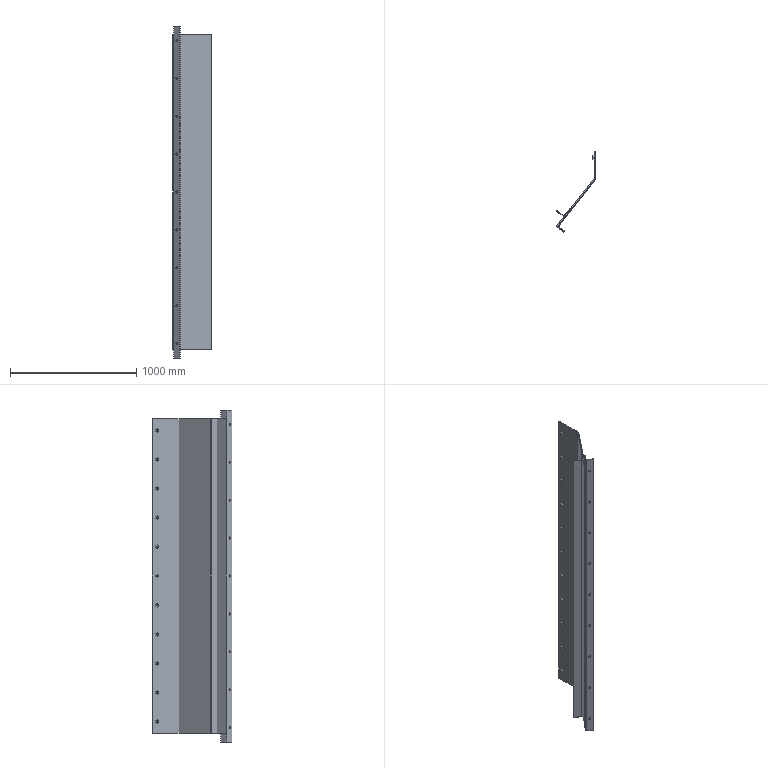Part | STEP file | Front baffle_Default<As machined> | 14 solids | 188 faces | box 304.499 x 630.195 x 2626 mm | volume 17251422 mm3 | plane 116 | cylinder 72 | commonest cylinder face diameters 18 x41 14 x23 3.333 x6 4 x1 20 x1